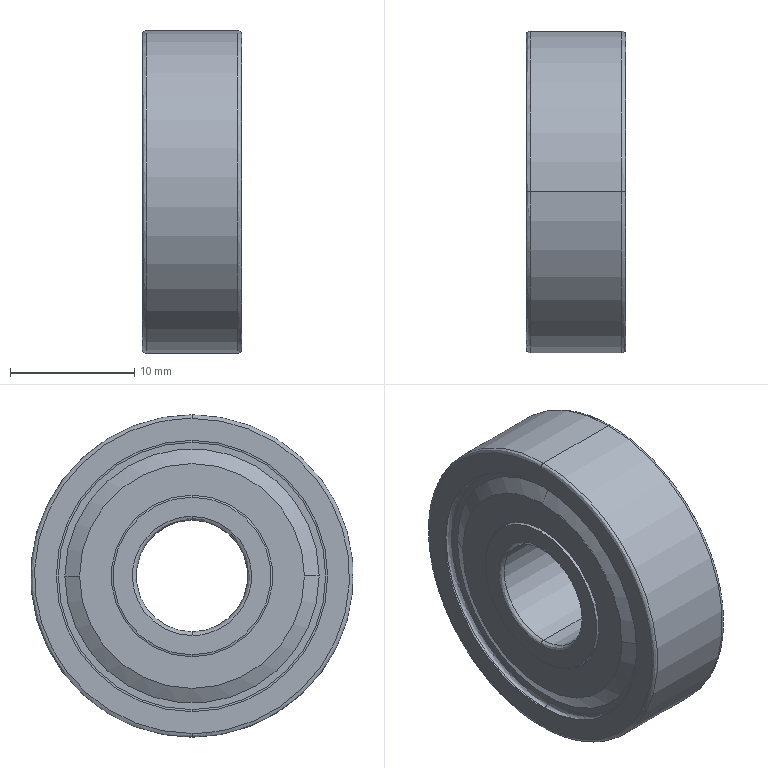Part | STEP file | BAF629ZZ-E | 1 solid | 70 faces | box 8 x 26 x 26 mm | volume 3194 mm3 | cylinder 24 | spline 20 | plane 14 | cone 12 | commonest cylinder face diameters 12.72 x4 13.02 x4 14 x4 21 x4 21.87 x4 9 x2